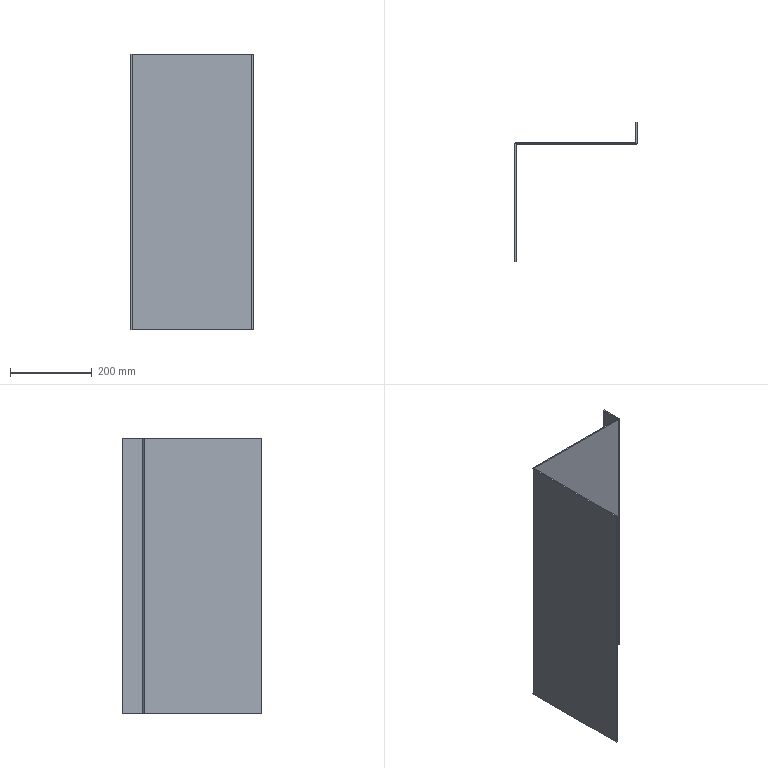Part | STEP file | E3-Metering stair tread 1-125 | 1 solid | 14 faces | box 299 x 340 x 674 mm | volume 1281653 mm3 | plane 10 | cylinder 4 | commonest cylinder face diameters 2 x2 8 x2
STEP:
#1=CARTESIAN_POINT('',(0.,0.,0.));
#2=DIRECTION('',(0.,0.,1.));
#3=DIRECTION('',(1.,0.,0.));
#4=AXIS2_PLACEMENT_3D('',#1,#2,#3);
#5=CARTESIAN_POINT('',(3.,1.,337.));
#6=VERTEX_POINT('',#5);
#7=CARTESIAN_POINT('',(3.,50.,337.));
#8=VERTEX_POINT('',#7);
#9=CARTESIAN_POINT('',(3.,1.,337.));
#10=DIRECTION('',(0.,1.,0.));
#11=VECTOR('',#10,1.);
#12=LINE('',#9,#11);
#13=CARTESIAN_POINT('',(3.,1.,-337.));
#14=DIRECTION('',(-1.,0.,0.));
#15=DIRECTION('',(0.,0.,-1.));
#16=AXIS2_PLACEMENT_3D('',#13,#14,#15);
#17=PLANE('',#16);
#18=CARTESIAN_POINT('',(-674.,0.));
#19=DIRECTION('',(0.,-1.));
#20=VECTOR('',#19,1.);
#21=LINE('',#18,#20);
#22=(GEOMETRIC_REPRESENTATION_CONTEXT(2)PARAMETRIC_REPRESENTATION_CONTEXT()REPRESENTATION_CONTEXT('',''));
#23=DEFINITIONAL_REPRESENTATION('',(#21),#22);
#24=PCURVE('',#17,#23);
#25=CARTESIAN_POINT('',(-1.,1.,337.));
#26=DIRECTION('',(0.,0.,-1.));
#27=DIRECTION('',(1.,0.,0.));
#28=AXIS2_PLACEMENT_3D('',#25,#26,#27);
#29=PLANE('',#28);
#30=CARTESIAN_POINT('',(4.,0.));
#31=DIRECTION('',(0.,-1.));
#32=VECTOR('',#31,1.);
#33=LINE('',#30,#32);
#34=(GEOMETRIC_REPRESENTATION_CONTEXT(2)PARAMETRIC_REPRESENTATION_CONTEXT()REPRESENTATION_CONTEXT('',''));
#35=DEFINITIONAL_REPRESENTATION('',(#33),#34);
#36=PCURVE('',#29,#35);
#37=SURFACE_CURVE('',#12,(#24,#36),.PCURVE_S1.);
#38=EDGE_CURVE('',#6,#8,#37,.T.);
#39=ORIENTED_EDGE('',*,*,#38,.F.);
#40=CARTESIAN_POINT('',(3.,1.,-337.));
#41=VERTEX_POINT('',#40);
#42=CARTESIAN_POINT('',(3.,1.,-337.));
#43=DIRECTION('',(0.,0.,1.));
#44=VECTOR('',#43,1.);
#45=LINE('',#42,#44);
#46=CARTESIAN_POINT('',(0.,0.));
#47=DIRECTION('',(-1.,0.));
#48=VECTOR('',#47,1.);
#49=LINE('',#46,#48);
#50=(GEOMETRIC_REPRESENTATION_CONTEXT(2)PARAMETRIC_REPRESENTATION_CONTEXT()REPRESENTATION_CONTEXT('',''));
#51=DEFINITIONAL_REPRESENTATION('',(#49),#50);
#52=PCURVE('',#17,#51);
#53=CARTESIAN_POINT('',(-1.,1.,-337.));
#54=DIRECTION('',(0.,0.,1.));
#55=DIRECTION('',(-1.,0.,0.));
#56=AXIS2_PLACEMENT_3D('',#53,#54,#55);
#57=CYLINDRICAL_SURFACE('',#56,4.);
#58=CARTESIAN_POINT('',(3.142,0.));
#59=DIRECTION('',(0.,1.));
#60=VECTOR('',#59,1.);
#61=LINE('',#58,#60);
#62=(GEOMETRIC_REPRESENTATION_CONTEXT(2)PARAMETRIC_REPRESENTATION_CONTEXT()REPRESENTATION_CONTEXT('',''));
#63=DEFINITIONAL_REPRESENTATION('',(#61),#62);
#64=PCURVE('',#57,#63);
#65=SURFACE_CURVE('',#45,(#52,#64),.PCURVE_S1.);
#66=EDGE_CURVE('',#41,#6,#65,.T.);
#67=ORIENTED_EDGE('',*,*,#66,.F.);
#68=CARTESIAN_POINT('',(3.,50.,-337.));
#69=VERTEX_POINT('',#68);
#70=CARTESIAN_POINT('',(3.,1.,-337.));
#71=DIRECTION('',(0.,1.,0.));
#72=VECTOR('',#71,1.);
#73=LINE('',#70,#72);
#74=CARTESIAN_POINT('',(0.,0.));
#75=DIRECTION('',(0.,-1.));
#76=VECTOR('',#75,1.);
#77=LINE('',#74,#76);
#78=(GEOMETRIC_REPRESENTATION_CONTEXT(2)PARAMETRIC_REPRESENTATION_CONTEXT()REPRESENTATION_CONTEXT('',''));
#79=DEFINITIONAL_REPRESENTATION('',(#77),#78);
#80=PCURVE('',#17,#79);
#81=CARTESIAN_POINT('',(-1.,1.,-337.));
#82=DIRECTION('',(0.,0.,-1.));
#83=DIRECTION('',(1.,0.,0.));
#84=AXIS2_PLACEMENT_3D('',#81,#82,#83);
#85=PLANE('',#84);
#86=CARTESIAN_POINT('',(4.,0.));
#87=DIRECTION('',(0.,-1.));
#88=VECTOR('',#87,1.);
#89=LINE('',#86,#88);
#90=(GEOMETRIC_REPRESENTATION_CONTEXT(2)PARAMETRIC_REPRESENTATION_CONTEXT()REPRESENTATION_CONTEXT('',''));
#91=DEFINITIONAL_REPRESENTATION('',(#89),#90);
#92=PCURVE('',#85,#91);
#93=SURFACE_CURVE('',#73,(#80,#92),.PCURVE_S1.);
#94=EDGE_CURVE('',#41,#69,#93,.T.);
#95=ORIENTED_EDGE('',*,*,#94,.T.);
#96=CARTESIAN_POINT('',(3.,50.,-337.));
#97=DIRECTION('',(0.,0.,1.));
#98=VECTOR('',#97,1.);
#99=LINE('',#96,#98);
#100=CARTESIAN_POINT('',(0.,-49.));
#101=DIRECTION('',(-1.,0.));
#102=VECTOR('',#101,1.);
#103=LINE('',#100,#102);
#104=(GEOMETRIC_REPRESENTATION_CONTEXT(2)PARAMETRIC_REPRESENTATION_CONTEXT()REPRESENTATION_CONTEXT('',''));
#105=DEFINITIONAL_REPRESENTATION('',(#103),#104);
#106=PCURVE('',#17,#105);
#107=CARTESIAN_POINT('',(0.,50.,-337.));
#108=DIRECTION('',(0.,1.,0.));
#109=DIRECTION('',(0.,0.,-1.));
#110=AXIS2_PLACEMENT_3D('',#107,#108,#109);
#111=PLANE('',#110);
#112=CARTESIAN_POINT('',(0.,-3.));
#113=DIRECTION('',(-1.,0.));
#114=VECTOR('',#113,1.);
#115=LINE('',#112,#114);
#116=(GEOMETRIC_REPRESENTATION_CONTEXT(2)PARAMETRIC_REPRESENTATION_CONTEXT()REPRESENTATION_CONTEXT('',''));
#117=DEFINITIONAL_REPRESENTATION('',(#115),#116);
#118=PCURVE('',#111,#117);
#119=SURFACE_CURVE('',#99,(#106,#118),.PCURVE_S1.);
#120=EDGE_CURVE('',#69,#8,#119,.T.);
#121=ORIENTED_EDGE('',*,*,#120,.T.);
#122=EDGE_LOOP('',(#39,#67,#95,#121));
#123=FACE_BOUND('',#122,.T.);
#124=ADVANCED_FACE('',(#123),#17,.F.);
#125=CARTESIAN_POINT('',(0.,50.,337.));
#126=VERTEX_POINT('',#125);
#127=CARTESIAN_POINT('',(0.,50.,337.));
#128=DIRECTION('',(1.,0.,0.));
#129=VECTOR('',#128,1.);
#130=LINE('',#127,#129);
#131=CARTESIAN_POINT('',(-674.,0.));
#132=DIRECTION('',(0.,-1.));
#133=VECTOR('',#132,1.);
#134=LINE('',#131,#133);
#135=(GEOMETRIC_REPRESENTATION_CONTEXT(2)PARAMETRIC_REPRESENTATION_CONTEXT()REPRESENTATION_CONTEXT('',''));
#136=DEFINITIONAL_REPRESENTATION('',(#134),#135);
#137=PCURVE('',#111,#136);
#138=CARTESIAN_POINT('',(1.,-49.));
#139=DIRECTION('',(1.,0.));
#140=VECTOR('',#139,1.);
#141=LINE('',#138,#140);
#142=(GEOMETRIC_REPRESENTATION_CONTEXT(2)PARAMETRIC_REPRESENTATION_CONTEXT()REPRESENTATION_CONTEXT('',''));
#143=DEFINITIONAL_REPRESENTATION('',(#141),#142);
#144=PCURVE('',#29,#143);
#145=SURFACE_CURVE('',#130,(#137,#144),.PCURVE_S1.);
#146=EDGE_CURVE('',#126,#8,#145,.T.);
#147=ORIENTED_EDGE('',*,*,#146,.T.);
#148=ORIENTED_EDGE('',*,*,#120,.F.);
#149=CARTESIAN_POINT('',(0.,50.,-337.));
#150=VERTEX_POINT('',#149);
#151=CARTESIAN_POINT('',(0.,50.,-337.));
#152=DIRECTION('',(1.,0.,0.));
#153=VECTOR('',#152,1.);
#154=LINE('',#151,#153);
#155=CARTESIAN_POINT('',(0.,0.));
#156=DIRECTION('',(0.,-1.));
#157=VECTOR('',#156,1.);
#158=LINE('',#155,#157);
#159=(GEOMETRIC_REPRESENTATION_CONTEXT(2)PARAMETRIC_REPRESENTATION_CONTEXT()REPRESENTATION_CONTEXT('',''));
#160=DEFINITIONAL_REPRESENTATION('',(#158),#159);
#161=PCURVE('',#111,#160);
#162=CARTESIAN_POINT('',(1.,-49.));
#163=DIRECTION('',(1.,0.));
#164=VECTOR('',#163,1.);
#165=LINE('',#162,#164);
#166=(GEOMETRIC_REPRESENTATION_CONTEXT(2)PARAMETRIC_REPRESENTATION_CONTEXT()REPRESENTATION_CONTEXT('',''));
#167=DEFINITIONAL_REPRESENTATION('',(#165),#166);
#168=PCURVE('',#85,#167);
#169=SURFACE_CURVE('',#154,(#161,#168),.PCURVE_S1.);
#170=EDGE_CURVE('',#150,#69,#169,.T.);
#171=ORIENTED_EDGE('',*,*,#170,.F.);
#172=CARTESIAN_POINT('',(0.,50.,-337.));
#173=DIRECTION('',(0.,0.,1.));
#174=VECTOR('',#173,1.);
#175=LINE('',#172,#174);
#176=CARTESIAN_POINT('',(0.,0.));
#177=DIRECTION('',(-1.,0.));
#178=VECTOR('',#177,1.);
#179=LINE('',#176,#178);
#180=(GEOMETRIC_REPRESENTATION_CONTEXT(2)PARAMETRIC_REPRESENTATION_CONTEXT()REPRESENTATION_CONTEXT('',''));
#181=DEFINITIONAL_REPRESENTATION('',(#179),#180);
#182=PCURVE('',#111,#181);
#183=CARTESIAN_POINT('',(0.,1.,-337.));
#184=DIRECTION('',(-1.,0.,0.));
#185=DIRECTION('',(0.,0.,-1.));
#186=AXIS2_PLACEMENT_3D('',#183,#184,#185);
#187=PLANE('',#186);
#188=CARTESIAN_POINT('',(0.,-49.));
#189=DIRECTION('',(-1.,0.));
#190=VECTOR('',#189,1.);
#191=LINE('',#188,#190);
#192=(GEOMETRIC_REPRESENTATION_CONTEXT(2)PARAMETRIC_REPRESENTATION_CONTEXT()REPRESENTATION_CONTEXT('',''));
#193=DEFINITIONAL_REPRESENTATION('',(#191),#192);
#194=PCURVE('',#187,#193);
#195=SURFACE_CURVE('',#175,(#182,#194),.PCURVE_S1.);
#196=EDGE_CURVE('',#150,#126,#195,.T.);
#197=ORIENTED_EDGE('',*,*,#196,.T.);
#198=EDGE_LOOP('',(#147,#148,#171,#197));
#199=FACE_BOUND('',#198,.T.);
#200=ADVANCED_FACE('',(#199),#111,.T.);
#201=CARTESIAN_POINT('',(0.,1.,337.));
#202=VERTEX_POINT('',#201);
#203=CARTESIAN_POINT('',(0.,1.,337.));
#204=DIRECTION('',(0.,1.,0.));
#205=VECTOR('',#204,1.);
#206=LINE('',#203,#205);
#207=CARTESIAN_POINT('',(-674.,0.));
#208=DIRECTION('',(0.,-1.));
#209=VECTOR('',#208,1.);
#210=LINE('',#207,#209);
#211=(GEOMETRIC_REPRESENTATION_CONTEXT(2)PARAMETRIC_REPRESENTATION_CONTEXT()REPRESENTATION_CONTEXT('',''));
#212=DEFINITIONAL_REPRESENTATION('',(#210),#211);
#213=PCURVE('',#187,#212);
#214=CARTESIAN_POINT('',(1.,0.));
#215=DIRECTION('',(0.,-1.));
#216=VECTOR('',#215,1.);
#217=LINE('',#214,#216);
#218=(GEOMETRIC_REPRESENTATION_CONTEXT(2)PARAMETRIC_REPRESENTATION_CONTEXT()REPRESENTATION_CONTEXT('',''));
#219=DEFINITIONAL_REPRESENTATION('',(#217),#218);
#220=PCURVE('',#29,#219);
#221=SURFACE_CURVE('',#206,(#213,#220),.PCURVE_S1.);
#222=EDGE_CURVE('',#202,#126,#221,.T.);
#223=ORIENTED_EDGE('',*,*,#222,.T.);
#224=ORIENTED_EDGE('',*,*,#196,.F.);
#225=CARTESIAN_POINT('',(0.,1.,-337.));
#226=VERTEX_POINT('',#225);
#227=CARTESIAN_POINT('',(0.,1.,-337.));
#228=DIRECTION('',(0.,1.,0.));
#229=VECTOR('',#228,1.);
#230=LINE('',#227,#229);
#231=CARTESIAN_POINT('',(0.,0.));
#232=DIRECTION('',(0.,-1.));
#233=VECTOR('',#232,1.);
#234=LINE('',#231,#233);
#235=(GEOMETRIC_REPRESENTATION_CONTEXT(2)PARAMETRIC_REPRESENTATION_CONTEXT()REPRESENTATION_CONTEXT('',''));
#236=DEFINITIONAL_REPRESENTATION('',(#234),#235);
#237=PCURVE('',#187,#236);
#238=CARTESIAN_POINT('',(1.,0.));
#239=DIRECTION('',(0.,-1.));
#240=VECTOR('',#239,1.);
#241=LINE('',#238,#240);
#242=(GEOMETRIC_REPRESENTATION_CONTEXT(2)PARAMETRIC_REPRESENTATION_CONTEXT()REPRESENTATION_CONTEXT('',''));
#243=DEFINITIONAL_REPRESENTATION('',(#241),#242);
#244=PCURVE('',#85,#243);
#245=SURFACE_CURVE('',#230,(#237,#244),.PCURVE_S1.);
#246=EDGE_CURVE('',#226,#150,#245,.T.);
#247=ORIENTED_EDGE('',*,*,#246,.F.);
#248=CARTESIAN_POINT('',(0.,1.,-337.));
#249=DIRECTION('',(0.,0.,1.));
#250=VECTOR('',#249,1.);
#251=LINE('',#248,#250);
#252=CARTESIAN_POINT('',(0.,0.));
#253=DIRECTION('',(-1.,0.));
#254=VECTOR('',#253,1.);
#255=LINE('',#252,#254);
#256=(GEOMETRIC_REPRESENTATION_CONTEXT(2)PARAMETRIC_REPRESENTATION_CONTEXT()REPRESENTATION_CONTEXT('',''));
#257=DEFINITIONAL_REPRESENTATION('',(#255),#256);
#258=PCURVE('',#187,#257);
#259=CARTESIAN_POINT('',(-1.,1.,-337.));
#260=DIRECTION('',(0.,0.,1.));
#261=DIRECTION('',(-1.,0.,0.));
#262=AXIS2_PLACEMENT_3D('',#259,#260,#261);
#263=CYLINDRICAL_SURFACE('',#262,1.);
#264=CARTESIAN_POINT('',(3.142,0.));
#265=DIRECTION('',(0.,1.));
#266=VECTOR('',#265,1.);
#267=LINE('',#264,#266);
#268=(GEOMETRIC_REPRESENTATION_CONTEXT(2)PARAMETRIC_REPRESENTATION_CONTEXT()REPRESENTATION_CONTEXT('',''));
#269=DEFINITIONAL_REPRESENTATION('',(#267),#268);
#270=PCURVE('',#263,#269);
#271=SURFACE_CURVE('',#251,(#258,#270),.PCURVE_S1.);
#272=EDGE_CURVE('',#226,#202,#271,.T.);
#273=ORIENTED_EDGE('',*,*,#272,.T.);
#274=EDGE_LOOP('',(#223,#224,#247,#273));
#275=FACE_BOUND('',#274,.T.);
#276=ADVANCED_FACE('',(#275),#187,.T.);
#277=CARTESIAN_POINT('',(-1.,0.,-337.));
#278=VERTEX_POINT('',#277);
#279=CARTESIAN_POINT('',(-1.,0.,337.));
#280=VERTEX_POINT('',#279);
#281=CARTESIAN_POINT('',(-1.,0.,-337.));
#282=DIRECTION('',(0.,0.,1.));
#283=VECTOR('',#282,1.);
#284=LINE('',#281,#283);
#285=CARTESIAN_POINT('',(1.571,0.));
#286=DIRECTION('',(0.,1.));
#287=VECTOR('',#286,1.);
#288=LINE('',#285,#287);
#289=(GEOMETRIC_REPRESENTATION_CONTEXT(2)PARAMETRIC_REPRESENTATION_CONTEXT()REPRESENTATION_CONTEXT('',''));
#290=DEFINITIONAL_REPRESENTATION('',(#288),#289);
#291=PCURVE('',#263,#290);
#292=CARTESIAN_POINT('',(-292.,0.,-337.));
#293=DIRECTION('',(0.,1.,0.));
#294=DIRECTION('',(0.,0.,-1.));
#295=AXIS2_PLACEMENT_3D('',#292,#293,#294);
#296=PLANE('',#295);
#297=CARTESIAN_POINT('',(0.,-291.));
#298=DIRECTION('',(-1.,0.));
#299=VECTOR('',#298,1.);
#300=LINE('',#297,#299);
#301=(GEOMETRIC_REPRESENTATION_CONTEXT(2)PARAMETRIC_REPRESENTATION_CONTEXT()REPRESENTATION_CONTEXT('',''));
#302=DEFINITIONAL_REPRESENTATION('',(#300),#301);
#303=PCURVE('',#296,#302);
#304=SURFACE_CURVE('',#284,(#291,#303),.PCURVE_S1.);
#305=EDGE_CURVE('',#278,#280,#304,.T.);
#306=ORIENTED_EDGE('',*,*,#305,.F.);
#307=CARTESIAN_POINT('',(-1.,1.,-337.));
#308=DIRECTION('',(0.,0.,1.));
#309=DIRECTION('',(1.,0.,0.));
#310=AXIS2_PLACEMENT_3D('',#307,#308,#309);
#311=CIRCLE('',#310,1.);
#312=CARTESIAN_POINT('',(-3.142,0.));
#313=DIRECTION('',(1.,0.));
#314=VECTOR('',#313,1.);
#315=LINE('',#312,#314);
#316=(GEOMETRIC_REPRESENTATION_CONTEXT(2)PARAMETRIC_REPRESENTATION_CONTEXT()REPRESENTATION_CONTEXT('',''));
#317=DEFINITIONAL_REPRESENTATION('',(#315),#316);
#318=PCURVE('',#263,#317);
#319=CARTESIAN_POINT('',(1.,0.));
#320=CARTESIAN_POINT('',(1.,-1.732));
#321=CARTESIAN_POINT('',(-0.5,-0.866));
#322=CARTESIAN_POINT('',(-2.,0.));
#323=CARTESIAN_POINT('',(-0.5,0.866));
#324=CARTESIAN_POINT('',(1.,1.732));
#325=CARTESIAN_POINT('',(1.,0.));
#326=(BOUNDED_CURVE()B_SPLINE_CURVE(2,(#319,#320,#321,#322,#323,#324,#325),.UNSPECIFIED.,.T.,.F.)B_SPLINE_CURVE_WITH_KNOTS((1,2,2,2,2,1),(-2.094,0.,2.094,4.189,6.283,8.378),.UNSPECIFIED.)CURVE()GEOMETRIC_REPRESENTATION_ITEM()RATIONAL_B_SPLINE_CURVE((1.,0.5,1.,0.5,1.,0.5,1.))REPRESENTATION_ITEM(''));
#327=(GEOMETRIC_REPRESENTATION_CONTEXT(2)PARAMETRIC_REPRESENTATION_CONTEXT()REPRESENTATION_CONTEXT('',''));
#328=DEFINITIONAL_REPRESENTATION('',(#326),#327);
#329=PCURVE('',#85,#328);
#330=SURFACE_CURVE('',#311,(#318,#329),.PCURVE_S1.);
#331=EDGE_CURVE('',#278,#226,#330,.T.);
#332=ORIENTED_EDGE('',*,*,#331,.T.);
#333=ORIENTED_EDGE('',*,*,#272,.T.);
#334=CARTESIAN_POINT('',(-1.,1.,337.));
#335=DIRECTION('',(0.,0.,1.));
#336=DIRECTION('',(1.,0.,0.));
#337=AXIS2_PLACEMENT_3D('',#334,#335,#336);
#338=CIRCLE('',#337,1.);
#339=CARTESIAN_POINT('',(-3.142,674.));
#340=DIRECTION('',(1.,0.));
#341=VECTOR('',#340,1.);
#342=LINE('',#339,#341);
#343=(GEOMETRIC_REPRESENTATION_CONTEXT(2)PARAMETRIC_REPRESENTATION_CONTEXT()REPRESENTATION_CONTEXT('',''));
#344=DEFINITIONAL_REPRESENTATION('',(#342),#343);
#345=PCURVE('',#263,#344);
#346=CARTESIAN_POINT('',(1.,0.));
#347=CARTESIAN_POINT('',(1.,-1.732));
#348=CARTESIAN_POINT('',(-0.5,-0.866));
#349=CARTESIAN_POINT('',(-2.,0.));
#350=CARTESIAN_POINT('',(-0.5,0.866));
#351=CARTESIAN_POINT('',(1.,1.732));
#352=CARTESIAN_POINT('',(1.,0.));
#353=(BOUNDED_CURVE()B_SPLINE_CURVE(2,(#346,#347,#348,#349,#350,#351,#352),.UNSPECIFIED.,.T.,.F.)B_SPLINE_CURVE_WITH_KNOTS((1,2,2,2,2,1),(-2.094,0.,2.094,4.189,6.283,8.378),.UNSPECIFIED.)CURVE()GEOMETRIC_REPRESENTATION_ITEM()RATIONAL_B_SPLINE_CURVE((1.,0.5,1.,0.5,1.,0.5,1.))REPRESENTATION_ITEM(''));
#354=(GEOMETRIC_REPRESENTATION_CONTEXT(2)PARAMETRIC_REPRESENTATION_CONTEXT()REPRESENTATION_CONTEXT('',''));
#355=DEFINITIONAL_REPRESENTATION('',(#353),#354);
#356=PCURVE('',#29,#355);
#357=SURFACE_CURVE('',#338,(#345,#356),.PCURVE_S1.);
#358=EDGE_CURVE('',#280,#202,#357,.T.);
#359=ORIENTED_EDGE('',*,*,#358,.F.);
#360=EDGE_LOOP('',(#306,#332,#333,#359));
#361=FACE_BOUND('',#360,.F.);
#362=ADVANCED_FACE('',(#361),#263,.F.);
#363=CARTESIAN_POINT('',(-292.,0.,337.));
#364=VERTEX_POINT('',#363);
#365=CARTESIAN_POINT('',(-292.,0.,337.));
#366=DIRECTION('',(1.,0.,0.));
#367=VECTOR('',#366,1.);
#368=LINE('',#365,#367);
#369=CARTESIAN_POINT('',(-674.,0.));
#370=DIRECTION('',(0.,-1.));
#371=VECTOR('',#370,1.);
#372=LINE('',#369,#371);
#373=(GEOMETRIC_REPRESENTATION_CONTEXT(2)PARAMETRIC_REPRESENTATION_CONTEXT()REPRESENTATION_CONTEXT('',''));
#374=DEFINITIONAL_REPRESENTATION('',(#372),#373);
#375=PCURVE('',#296,#374);
#376=CARTESIAN_POINT('',(-291.,1.));
#377=DIRECTION('',(1.,0.));
#378=VECTOR('',#377,1.);
#379=LINE('',#376,#378);
#380=(GEOMETRIC_REPRESENTATION_CONTEXT(2)PARAMETRIC_REPRESENTATION_CONTEXT()REPRESENTATION_CONTEXT('',''));
#381=DEFINITIONAL_REPRESENTATION('',(#379),#380);
#382=PCURVE('',#29,#381);
#383=SURFACE_CURVE('',#368,(#375,#382),.PCURVE_S1.);
#384=EDGE_CURVE('',#364,#280,#383,.T.);
#385=ORIENTED_EDGE('',*,*,#384,.T.);
#386=ORIENTED_EDGE('',*,*,#305,.F.);
#387=CARTESIAN_POINT('',(-292.,0.,-337.));
#388=VERTEX_POINT('',#387);
#389=CARTESIAN_POINT('',(-292.,0.,-337.));
#390=DIRECTION('',(1.,0.,0.));
#391=VECTOR('',#390,1.);
#392=LINE('',#389,#391);
#393=CARTESIAN_POINT('',(0.,0.));
#394=DIRECTION('',(0.,-1.));
#395=VECTOR('',#394,1.);
#396=LINE('',#393,#395);
#397=(GEOMETRIC_REPRESENTATION_CONTEXT(2)PARAMETRIC_REPRESENTATION_CONTEXT()REPRESENTATION_CONTEXT('',''));
#398=DEFINITIONAL_REPRESENTATION('',(#396),#397);
#399=PCURVE('',#296,#398);
#400=CARTESIAN_POINT('',(-291.,1.));
#401=DIRECTION('',(1.,0.));
#402=VECTOR('',#401,1.);
#403=LINE('',#400,#402);
#404=(GEOMETRIC_REPRESENTATION_CONTEXT(2)PARAMETRIC_REPRESENTATION_CONTEXT()REPRESENTATION_CONTEXT('',''));
#405=DEFINITIONAL_REPRESENTATION('',(#403),#404);
#406=PCURVE('',#85,#405);
#407=SURFACE_CURVE('',#392,(#399,#406),.PCURVE_S1.);
#408=EDGE_CURVE('',#388,#278,#407,.T.);
#409=ORIENTED_EDGE('',*,*,#408,.F.);
#410=CARTESIAN_POINT('',(-292.,0.,-337.));
#411=DIRECTION('',(0.,0.,1.));
#412=VECTOR('',#411,1.);
#413=LINE('',#410,#412);
#414=CARTESIAN_POINT('',(0.,0.));
#415=DIRECTION('',(-1.,0.));
#416=VECTOR('',#415,1.);
#417=LINE('',#414,#416);
#418=(GEOMETRIC_REPRESENTATION_CONTEXT(2)PARAMETRIC_REPRESENTATION_CONTEXT()REPRESENTATION_CONTEXT('',''));
#419=DEFINITIONAL_REPRESENTATION('',(#417),#418);
#420=PCURVE('',#296,#419);
#421=CARTESIAN_POINT('',(-292.,-4.,-337.));
#422=DIRECTION('',(0.,0.,1.));
#423=DIRECTION('',(-1.,0.,0.));
#424=AXIS2_PLACEMENT_3D('',#421,#422,#423);
#425=CYLINDRICAL_SURFACE('',#424,4.);
#426=CARTESIAN_POINT('',(4.712,0.));
#427=DIRECTION('',(0.,1.));
#428=VECTOR('',#427,1.);
#429=LINE('',#426,#428);
#430=(GEOMETRIC_REPRESENTATION_CONTEXT(2)PARAMETRIC_REPRESENTATION_CONTEXT()REPRESENTATION_CONTEXT('',''));
#431=DEFINITIONAL_REPRESENTATION('',(#429),#430);
#432=PCURVE('',#425,#431);
#433=SURFACE_CURVE('',#413,(#420,#432),.PCURVE_S1.);
#434=EDGE_CURVE('',#388,#364,#433,.T.);
#435=ORIENTED_EDGE('',*,*,#434,.T.);
#436=EDGE_LOOP('',(#385,#386,#409,#435));
#437=FACE_BOUND('',#436,.T.);
#438=ADVANCED_FACE('',(#437),#296,.T.);
#439=CARTESIAN_POINT('',(-296.,-4.,337.));
#440=VERTEX_POINT('',#439);
#441=CARTESIAN_POINT('',(-292.,-4.,337.));
#442=DIRECTION('',(0.,0.,-1.));
#443=DIRECTION('',(1.,0.,0.));
#444=AXIS2_PLACEMENT_3D('',#441,#442,#443);
#445=CIRCLE('',#444,4.);
#446=CARTESIAN_POINT('',(9.425,674.));
#447=DIRECTION('',(-1.,0.));
#448=VECTOR('',#447,1.);
#449=LINE('',#446,#448);
#450=(GEOMETRIC_REPRESENTATION_CONTEXT(2)PARAMETRIC_REPRESENTATION_CONTEXT()REPRESENTATION_CONTEXT('',''));
#451=DEFINITIONAL_REPRESENTATION('',(#449),#450);
#452=PCURVE('',#425,#451);
#453=CARTESIAN_POINT('',(-291.,5.));
#454=DIRECTION('',(1.,0.));
#455=AXIS2_PLACEMENT_2D('',#453,#454);
#456=CIRCLE('',#455,4.);
#457=(GEOMETRIC_REPRESENTATION_CONTEXT(2)PARAMETRIC_REPRESENTATION_CONTEXT()REPRESENTATION_CONTEXT('',''));
#458=DEFINITIONAL_REPRESENTATION('',(#456),#457);
#459=PCURVE('',#29,#458);
#460=SURFACE_CURVE('',#445,(#452,#459),.PCURVE_S1.);
#461=EDGE_CURVE('',#440,#364,#460,.T.);
#462=ORIENTED_EDGE('',*,*,#461,.T.);
#463=ORIENTED_EDGE('',*,*,#434,.F.);
#464=CARTESIAN_POINT('',(-296.,-4.,-337.));
#465=VERTEX_POINT('',#464);
#466=CARTESIAN_POINT('',(-292.,-4.,-337.));
#467=DIRECTION('',(0.,0.,-1.));
#468=DIRECTION('',(1.,0.,0.));
#469=AXIS2_PLACEMENT_3D('',#466,#467,#468);
#470=CIRCLE('',#469,4.);
#471=CARTESIAN_POINT('',(9.425,0.));
#472=DIRECTION('',(-1.,0.));
#473=VECTOR('',#472,1.);
#474=LINE('',#471,#473);
#475=(GEOMETRIC_REPRESENTATION_CONTEXT(2)PARAMETRIC_REPRESENTATION_CONTEXT()REPRESENTATION_CONTEXT('',''));
#476=DEFINITIONAL_REPRESENTATION('',(#474),#475);
#477=PCURVE('',#425,#476);
#478=CARTESIAN_POINT('',(-291.,5.));
#479=DIRECTION('',(1.,0.));
#480=AXIS2_PLACEMENT_2D('',#478,#479);
#481=CIRCLE('',#480,4.);
#482=(GEOMETRIC_REPRESENTATION_CONTEXT(2)PARAMETRIC_REPRESENTATION_CONTEXT()REPRESENTATION_CONTEXT('',''));
#483=DEFINITIONAL_REPRESENTATION('',(#481),#482);
#484=PCURVE('',#85,#483);
#485=SURFACE_CURVE('',#470,(#477,#484),.PCURVE_S1.);
#486=EDGE_CURVE('',#465,#388,#485,.T.);
#487=ORIENTED_EDGE('',*,*,#486,.F.);
#488=CARTESIAN_POINT('',(-296.,-4.,-337.));
#489=DIRECTION('',(0.,0.,1.));
#490=VECTOR('',#489,1.);
#491=LINE('',#488,#490);
#492=CARTESIAN_POINT('',(6.283,0.));
#493=DIRECTION('',(0.,1.));
#494=VECTOR('',#493,1.);
#495=LINE('',#492,#494);
#496=(GEOMETRIC_REPRESENTATION_CONTEXT(2)PARAMETRIC_REPRESENTATION_CONTEXT()REPRESENTATION_CONTEXT('',''));
#497=DEFINITIONAL_REPRESENTATION('',(#495),#496);
#498=PCURVE('',#425,#497);
#499=CARTESIAN_POINT('',(-296.,-4.,-337.));
#500=DIRECTION('',(-1.,0.,0.));
#501=DIRECTION('',(0.,0.,-1.));
#502=AXIS2_PLACEMENT_3D('',#499,#500,#501);
#503=PLANE('',#502);
#504=CARTESIAN_POINT('',(0.,0.));
#505=DIRECTION('',(-1.,0.));
#506=VECTOR('',#505,1.);
#507=LINE('',#504,#506);
#508=(GEOMETRIC_REPRESENTATION_CONTEXT(2)PARAMETRIC_REPRESENTATION_CONTEXT()REPRESENTATION_CONTEXT('',''));
#509=DEFINITIONAL_REPRESENTATION('',(#507),#508);
#510=PCURVE('',#503,#509);
#511=SURFACE_CURVE('',#491,(#498,#510),.PCURVE_S1.);
#512=EDGE_CURVE('',#465,#440,#511,.T.);
#513=ORIENTED_EDGE('',*,*,#512,.T.);
#514=EDGE_LOOP('',(#462,#463,#487,#513));
#515=FACE_BOUND('',#514,.T.);
#516=ADVANCED_FACE('',(#515),#425,.T.);
#517=CARTESIAN_POINT('',(-296.,-290.,337.));
#518=VERTEX_POINT('',#517);
#519=CARTESIAN_POINT('',(-296.,-4.,337.));
#520=DIRECTION('',(0.,1.,0.));
#521=VECTOR('',#520,1.);
#522=LINE('',#519,#521);
#523=CARTESIAN_POINT('',(-674.,0.));
#524=DIRECTION('',(0.,-1.));
#525=VECTOR('',#524,1.);
#526=LINE('',#523,#525);
#527=(GEOMETRIC_REPRESENTATION_CONTEXT(2)PARAMETRIC_REPRESENTATION_CONTEXT()REPRESENTATION_CONTEXT('',''));
#528=DEFINITIONAL_REPRESENTATION('',(#526),#527);
#529=PCURVE('',#503,#528);
#530=CARTESIAN_POINT('',(-295.,5.));
#531=DIRECTION('',(0.,-1.));
#532=VECTOR('',#531,1.);
#533=LINE('',#530,#532);
#534=(GEOMETRIC_REPRESENTATION_CONTEXT(2)PARAMETRIC_REPRESENTATION_CONTEXT()REPRESENTATION_CONTEXT('',''));
#535=DEFINITIONAL_REPRESENTATION('',(#533),#534);
#536=PCURVE('',#29,#535);
#537=SURFACE_CURVE('',#522,(#529,#536),.PCURVE_S1.);
#538=EDGE_CURVE('',#518,#440,#537,.T.);
#539=ORIENTED_EDGE('',*,*,#538,.T.);
#540=ORIENTED_EDGE('',*,*,#512,.F.);
#541=CARTESIAN_POINT('',(-296.,-290.,-337.));
#542=VERTEX_POINT('',#541);
#543=CARTESIAN_POINT('',(-296.,-4.,-337.));
#544=DIRECTION('',(0.,1.,0.));
#545=VECTOR('',#544,1.);
#546=LINE('',#543,#545);
#547=CARTESIAN_POINT('',(0.,0.));
#548=DIRECTION('',(0.,-1.));
#549=VECTOR('',#548,1.);
#550=LINE('',#547,#549);
#551=(GEOMETRIC_REPRESENTATION_CONTEXT(2)PARAMETRIC_REPRESENTATION_CONTEXT()REPRESENTATION_CONTEXT('',''));
#552=DEFINITIONAL_REPRESENTATION('',(#550),#551);
#553=PCURVE('',#503,#552);
#554=CARTESIAN_POINT('',(-295.,5.));
#555=DIRECTION('',(0.,-1.));
#556=VECTOR('',#555,1.);
#557=LINE('',#554,#556);
#558=(GEOMETRIC_REPRESENTATION_CONTEXT(2)PARAMETRIC_REPRESENTATION_CONTEXT()REPRESENTATION_CONTEXT('',''));
#559=DEFINITIONAL_REPRESENTATION('',(#557),#558);
#560=PCURVE('',#85,#559);
#561=SURFACE_CURVE('',#546,(#553,#560),.PCURVE_S1.);
#562=EDGE_CURVE('',#542,#465,#561,.T.);
#563=ORIENTED_EDGE('',*,*,#562,.F.);
#564=CARTESIAN_POINT('',(-296.,-290.,-337.));
#565=DIRECTION('',(0.,0.,1.));
#566=VECTOR('',#565,1.);
#567=LINE('',#564,#566);
#568=CARTESIAN_POINT('',(0.,286.));
#569=DIRECTION('',(-1.,0.));
#570=VECTOR('',#569,1.);
#571=LINE('',#568,#570);
#572=(GEOMETRIC_REPRESENTATION_CONTEXT(2)PARAMETRIC_REPRESENTATION_CONTEXT()REPRESENTATION_CONTEXT('',''));
#573=DEFINITIONAL_REPRESENTATION('',(#571),#572);
#574=PCURVE('',#503,#573);
#575=CARTESIAN_POINT('',(-293.,-290.,-337.));
#576=DIRECTION('',(0.,-1.,0.));
#577=DIRECTION('',(0.,0.,1.));
#578=AXIS2_PLACEMENT_3D('',#575,#576,#577);
#579=PLANE('',#578);
#580=CARTESIAN_POINT('',(0.,3.));
#581=DIRECTION('',(1.,0.));
#582=VECTOR('',#581,1.);
#583=LINE('',#580,#582);
#584=(GEOMETRIC_REPRESENTATION_CONTEXT(2)PARAMETRIC_REPRESENTATION_CONTEXT()REPRESENTATION_CONTEXT('',''));
#585=DEFINITIONAL_REPRESENTATION('',(#583),#584);
#586=PCURVE('',#579,#585);
#587=SURFACE_CURVE('',#567,(#574,#586),.PCURVE_S1.);
#588=EDGE_CURVE('',#542,#518,#587,.T.);
#589=ORIENTED_EDGE('',*,*,#588,.T.);
#590=EDGE_LOOP('',(#539,#540,#563,#589));
#591=FACE_BOUND('',#590,.T.);
#592=ADVANCED_FACE('',(#591),#503,.T.);
#593=CARTESIAN_POINT('',(-293.,-290.,337.));
#594=VERTEX_POINT('',#593);
#595=CARTESIAN_POINT('',(-293.,-290.,337.));
#596=DIRECTION('',(-1.,0.,0.));
#597=VECTOR('',#596,1.);
#598=LINE('',#595,#597);
#599=CARTESIAN_POINT('',(674.,0.));
#600=DIRECTION('',(0.,1.));
#601=VECTOR('',#600,1.);
#602=LINE('',#599,#601);
#603=(GEOMETRIC_REPRESENTATION_CONTEXT(2)PARAMETRIC_REPRESENTATION_CONTEXT()REPRESENTATION_CONTEXT('',''));
#604=DEFINITIONAL_REPRESENTATION('',(#602),#603);
#605=PCURVE('',#579,#604);
#606=CARTESIAN_POINT('',(-292.,291.));
#607=DIRECTION('',(-1.,0.));
#608=VECTOR('',#607,1.);
#609=LINE('',#606,#608);
#610=(GEOMETRIC_REPRESENTATION_CONTEXT(2)PARAMETRIC_REPRESENTATION_CONTEXT()REPRESENTATION_CONTEXT('',''));
#611=DEFINITIONAL_REPRESENTATION('',(#609),#610);
#612=PCURVE('',#29,#611);
#613=SURFACE_CURVE('',#598,(#605,#612),.PCURVE_S1.);
#614=EDGE_CURVE('',#594,#518,#613,.T.);
#615=ORIENTED_EDGE('',*,*,#614,.T.);
#616=ORIENTED_EDGE('',*,*,#588,.F.);
#617=CARTESIAN_POINT('',(-293.,-290.,-337.));
#618=VERTEX_POINT('',#617);
#619=CARTESIAN_POINT('',(-293.,-290.,-337.));
#620=DIRECTION('',(-1.,0.,0.));
#621=VECTOR('',#620,1.);
#622=LINE('',#619,#621);
#623=CARTESIAN_POINT('',(0.,0.));
#624=DIRECTION('',(0.,1.));
#625=VECTOR('',#624,1.);
#626=LINE('',#623,#625);
#627=(GEOMETRIC_REPRESENTATION_CONTEXT(2)PARAMETRIC_REPRESENTATION_CONTEXT()REPRESENTATION_CONTEXT('',''));
#628=DEFINITIONAL_REPRESENTATION('',(#626),#627);
#629=PCURVE('',#579,#628);
#630=CARTESIAN_POINT('',(-292.,291.));
#631=DIRECTION('',(-1.,0.));
#632=VECTOR('',#631,1.);
#633=LINE('',#630,#632);
#634=(GEOMETRIC_REPRESENTATION_CONTEXT(2)PARAMETRIC_REPRESENTATION_CONTEXT()REPRESENTATION_CONTEXT('',''));
#635=DEFINITIONAL_REPRESENTATION('',(#633),#634);
#636=PCURVE('',#85,#635);
#637=SURFACE_CURVE('',#622,(#629,#636),.PCURVE_S1.);
#638=EDGE_CURVE('',#618,#542,#637,.T.);
#639=ORIENTED_EDGE('',*,*,#638,.F.);
#640=CARTESIAN_POINT('',(-293.,-290.,-337.));
#641=DIRECTION('',(0.,0.,1.));
#642=VECTOR('',#641,1.);
#643=LINE('',#640,#642);
#644=CARTESIAN_POINT('',(0.,0.));
#645=DIRECTION('',(1.,0.));
#646=VECTOR('',#645,1.);
#647=LINE('',#644,#646);
#648=(GEOMETRIC_REPRESENTATION_CONTEXT(2)PARAMETRIC_REPRESENTATION_CONTEXT()REPRESENTATION_CONTEXT('',''));
#649=DEFINITIONAL_REPRESENTATION('',(#647),#648);
#650=PCURVE('',#579,#649);
#651=CARTESIAN_POINT('',(-293.,-4.,-337.));
#652=DIRECTION('',(-1.,0.,0.));
#653=DIRECTION('',(0.,0.,-1.));
#654=AXIS2_PLACEMENT_3D('',#651,#652,#653);
#655=PLANE('',#654);
#656=CARTESIAN_POINT('',(0.,286.));
#657=DIRECTION('',(-1.,0.));
#658=VECTOR('',#657,1.);
#659=LINE('',#656,#658);
#660=(GEOMETRIC_REPRESENTATION_CONTEXT(2)PARAMETRIC_REPRESENTATION_CONTEXT()REPRESENTATION_CONTEXT('',''));
#661=DEFINITIONAL_REPRESENTATION('',(#659),#660);
#662=PCURVE('',#655,#661);
#663=SURFACE_CURVE('',#643,(#650,#662),.PCURVE_S1.);
#664=EDGE_CURVE('',#618,#594,#663,.T.);
#665=ORIENTED_EDGE('',*,*,#664,.T.);
#666=EDGE_LOOP('',(#615,#616,#639,#665));
#667=FACE_BOUND('',#666,.T.);
#668=ADVANCED_FACE('',(#667),#579,.T.);
#669=CARTESIAN_POINT('',(-293.,-4.,337.));
#670=VERTEX_POINT('',#669);
#671=CARTESIAN_POINT('',(-293.,-4.,337.));
#672=DIRECTION('',(0.,1.,0.));
#673=VECTOR('',#672,1.);
#674=LINE('',#671,#673);
#675=CARTESIAN_POINT('',(-674.,0.));
#676=DIRECTION('',(0.,-1.));
#677=VECTOR('',#676,1.);
#678=LINE('',#675,#677);
#679=(GEOMETRIC_REPRESENTATION_CONTEXT(2)PARAMETRIC_REPRESENTATION_CONTEXT()REPRESENTATION_CONTEXT('',''));
#680=DEFINITIONAL_REPRESENTATION('',(#678),#679);
#681=PCURVE('',#655,#680);
#682=CARTESIAN_POINT('',(-292.,5.));
#683=DIRECTION('',(0.,-1.));
#684=VECTOR('',#683,1.);
#685=LINE('',#682,#684);
#686=(GEOMETRIC_REPRESENTATION_CONTEXT(2)PARAMETRIC_REPRESENTATION_CONTEXT()REPRESENTATION_CONTEXT('',''));
#687=DEFINITIONAL_REPRESENTATION('',(#685),#686);
#688=PCURVE('',#29,#687);
#689=SURFACE_CURVE('',#674,(#681,#688),.PCURVE_S1.);
#690=EDGE_CURVE('',#594,#670,#689,.T.);
#691=ORIENTED_EDGE('',*,*,#690,.F.);
#692=ORIENTED_EDGE('',*,*,#664,.F.);
#693=CARTESIAN_POINT('',(-293.,-4.,-337.));
#694=VERTEX_POINT('',#693);
#695=CARTESIAN_POINT('',(-293.,-4.,-337.));
#696=DIRECTION('',(0.,1.,0.));
#697=VECTOR('',#696,1.);
#698=LINE('',#695,#697);
#699=CARTESIAN_POINT('',(0.,0.));
#700=DIRECTION('',(0.,-1.));
#701=VECTOR('',#700,1.);
#702=LINE('',#699,#701);
#703=(GEOMETRIC_REPRESENTATION_CONTEXT(2)PARAMETRIC_REPRESENTATION_CONTEXT()REPRESENTATION_CONTEXT('',''));
#704=DEFINITIONAL_REPRESENTATION('',(#702),#703);
#705=PCURVE('',#655,#704);
#706=CARTESIAN_POINT('',(-292.,5.));
#707=DIRECTION('',(0.,-1.));
#708=VECTOR('',#707,1.);
#709=LINE('',#706,#708);
#710=(GEOMETRIC_REPRESENTATION_CONTEXT(2)PARAMETRIC_REPRESENTATION_CONTEXT()REPRESENTATION_CONTEXT('',''));
#711=DEFINITIONAL_REPRESENTATION('',(#709),#710);
#712=PCURVE('',#85,#711);
#713=SURFACE_CURVE('',#698,(#705,#712),.PCURVE_S1.);
#714=EDGE_CURVE('',#618,#694,#713,.T.);
#715=ORIENTED_EDGE('',*,*,#714,.T.);
#716=CARTESIAN_POINT('',(-293.,-4.,-337.));
#717=DIRECTION('',(0.,0.,1.));
#718=VECTOR('',#717,1.);
#719=LINE('',#716,#718);
#720=CARTESIAN_POINT('',(0.,0.));
#721=DIRECTION('',(-1.,0.));
#722=VECTOR('',#721,1.);
#723=LINE('',#720,#722);
#724=(GEOMETRIC_REPRESENTATION_CONTEXT(2)PARAMETRIC_REPRESENTATION_CONTEXT()REPRESENTATION_CONTEXT('',''));
#725=DEFINITIONAL_REPRESENTATION('',(#723),#724);
#726=PCURVE('',#655,#725);
#727=CARTESIAN_POINT('',(-292.,-4.,-337.));
#728=DIRECTION('',(0.,0.,1.));
#729=DIRECTION('',(-1.,0.,0.));
#730=AXIS2_PLACEMENT_3D('',#727,#728,#729);
#731=CYLINDRICAL_SURFACE('',#730,1.);
#732=CARTESIAN_POINT('',(6.283,0.));
#733=DIRECTION('',(0.,1.));
#734=VECTOR('',#733,1.);
#735=LINE('',#732,#734);
#736=(GEOMETRIC_REPRESENTATION_CONTEXT(2)PARAMETRIC_REPRESENTATION_CONTEXT()REPRESENTATION_CONTEXT('',''));
#737=DEFINITIONAL_REPRESENTATION('',(#735),#736);
#738=PCURVE('',#731,#737);
#739=SURFACE_CURVE('',#719,(#726,#738),.PCURVE_S1.);
#740=EDGE_CURVE('',#694,#670,#739,.T.);
#741=ORIENTED_EDGE('',*,*,#740,.T.);
#742=EDGE_LOOP('',(#691,#692,#715,#741));
#743=FACE_BOUND('',#742,.T.);
#744=ADVANCED_FACE('',(#743),#655,.F.);
#745=CARTESIAN_POINT('',(-292.,-3.,-337.));
#746=VERTEX_POINT('',#745);
#747=CARTESIAN_POINT('',(-292.,-3.,337.));
#748=VERTEX_POINT('',#747);
#749=CARTESIAN_POINT('',(-292.,-3.,-337.));
#750=DIRECTION('',(0.,0.,1.));
#751=VECTOR('',#750,1.);
#752=LINE('',#749,#751);
#753=CARTESIAN_POINT('',(4.712,0.));
#754=DIRECTION('',(0.,1.));
#755=VECTOR('',#754,1.);
#756=LINE('',#753,#755);
#757=(GEOMETRIC_REPRESENTATION_CONTEXT(2)PARAMETRIC_REPRESENTATION_CONTEXT()REPRESENTATION_CONTEXT('',''));
#758=DEFINITIONAL_REPRESENTATION('',(#756),#757);
#759=PCURVE('',#731,#758);
#760=CARTESIAN_POINT('',(-292.,-3.,-337.));
#761=DIRECTION('',(0.,1.,0.));
#762=DIRECTION('',(0.,0.,-1.));
#763=AXIS2_PLACEMENT_3D('',#760,#761,#762);
#764=PLANE('',#763);
#765=CARTESIAN_POINT('',(0.,0.));
#766=DIRECTION('',(-1.,0.));
#767=VECTOR('',#766,1.);
#768=LINE('',#765,#767);
#769=(GEOMETRIC_REPRESENTATION_CONTEXT(2)PARAMETRIC_REPRESENTATION_CONTEXT()REPRESENTATION_CONTEXT('',''));
#770=DEFINITIONAL_REPRESENTATION('',(#768),#769);
#771=PCURVE('',#764,#770);
#772=SURFACE_CURVE('',#752,(#759,#771),.PCURVE_S1.);
#773=EDGE_CURVE('',#746,#748,#772,.T.);
#774=ORIENTED_EDGE('',*,*,#773,.F.);
#775=CARTESIAN_POINT('',(-292.,-4.,-337.));
#776=DIRECTION('',(0.,0.,-1.));
#777=DIRECTION('',(1.,0.,0.));
#778=AXIS2_PLACEMENT_3D('',#775,#776,#777);
#779=CIRCLE('',#778,1.);
#780=CARTESIAN_POINT('',(9.425,0.));
#781=DIRECTION('',(-1.,0.));
#782=VECTOR('',#781,1.);
#783=LINE('',#780,#782);
#784=(GEOMETRIC_REPRESENTATION_CONTEXT(2)PARAMETRIC_REPRESENTATION_CONTEXT()REPRESENTATION_CONTEXT('',''));
#785=DEFINITIONAL_REPRESENTATION('',(#783),#784);
#786=PCURVE('',#731,#785);
#787=CARTESIAN_POINT('',(-291.,5.));
#788=DIRECTION('',(1.,0.));
#789=AXIS2_PLACEMENT_2D('',#787,#788);
#790=CIRCLE('',#789,1.);
#791=(GEOMETRIC_REPRESENTATION_CONTEXT(2)PARAMETRIC_REPRESENTATION_CONTEXT()REPRESENTATION_CONTEXT('',''));
#792=DEFINITIONAL_REPRESENTATION('',(#790),#791);
#793=PCURVE('',#85,#792);
#794=SURFACE_CURVE('',#779,(#786,#793),.PCURVE_S1.);
#795=EDGE_CURVE('',#694,#746,#794,.T.);
#796=ORIENTED_EDGE('',*,*,#795,.F.);
#797=ORIENTED_EDGE('',*,*,#740,.T.);
#798=CARTESIAN_POINT('',(-292.,-4.,337.));
#799=DIRECTION('',(0.,0.,-1.));
#800=DIRECTION('',(1.,0.,0.));
#801=AXIS2_PLACEMENT_3D('',#798,#799,#800);
#802=CIRCLE('',#801,1.);
#803=CARTESIAN_POINT('',(9.425,674.));
#804=DIRECTION('',(-1.,0.));
#805=VECTOR('',#804,1.);
#806=LINE('',#803,#805);
#807=(GEOMETRIC_REPRESENTATION_CONTEXT(2)PARAMETRIC_REPRESENTATION_CONTEXT()REPRESENTATION_CONTEXT('',''));
#808=DEFINITIONAL_REPRESENTATION('',(#806),#807);
#809=PCURVE('',#731,#808);
#810=CARTESIAN_POINT('',(-291.,5.));
#811=DIRECTION('',(1.,0.));
#812=AXIS2_PLACEMENT_2D('',#810,#811);
#813=CIRCLE('',#812,1.);
#814=(GEOMETRIC_REPRESENTATION_CONTEXT(2)PARAMETRIC_REPRESENTATION_CONTEXT()REPRESENTATION_CONTEXT('',''));
#815=DEFINITIONAL_REPRESENTATION('',(#813),#814);
#816=PCURVE('',#29,#815);
#817=SURFACE_CURVE('',#802,(#809,#816),.PCURVE_S1.);
#818=EDGE_CURVE('',#670,#748,#817,.T.);
#819=ORIENTED_EDGE('',*,*,#818,.T.);
#820=EDGE_LOOP('',(#774,#796,#797,#819));
#821=FACE_BOUND('',#820,.F.);
#822=ADVANCED_FACE('',(#821),#731,.F.);
#823=CARTESIAN_POINT('',(-1.,-3.,337.));
#824=VERTEX_POINT('',#823);
#825=CARTESIAN_POINT('',(-292.,-3.,337.));
#826=DIRECTION('',(1.,0.,0.));
#827=VECTOR('',#826,1.);
#828=LINE('',#825,#827);
#829=CARTESIAN_POINT('',(-674.,0.));
#830=DIRECTION('',(0.,-1.));
#831=VECTOR('',#830,1.);
#832=LINE('',#829,#831);
#833=(GEOMETRIC_REPRESENTATION_CONTEXT(2)PARAMETRIC_REPRESENTATION_CONTEXT()REPRESENTATION_CONTEXT('',''));
#834=DEFINITIONAL_REPRESENTATION('',(#832),#833);
#835=PCURVE('',#764,#834);
#836=CARTESIAN_POINT('',(-291.,4.));
#837=DIRECTION('',(1.,0.));
#838=VECTOR('',#837,1.);
#839=LINE('',#836,#838);
#840=(GEOMETRIC_REPRESENTATION_CONTEXT(2)PARAMETRIC_REPRESENTATION_CONTEXT()REPRESENTATION_CONTEXT('',''));
#841=DEFINITIONAL_REPRESENTATION('',(#839),#840);
#842=PCURVE('',#29,#841);
#843=SURFACE_CURVE('',#828,(#835,#842),.PCURVE_S1.);
#844=EDGE_CURVE('',#748,#824,#843,.T.);
#845=ORIENTED_EDGE('',*,*,#844,.F.);
#846=ORIENTED_EDGE('',*,*,#773,.F.);
#847=CARTESIAN_POINT('',(-1.,-3.,-337.));
#848=VERTEX_POINT('',#847);
#849=CARTESIAN_POINT('',(-292.,-3.,-337.));
#850=DIRECTION('',(1.,0.,0.));
#851=VECTOR('',#850,1.);
#852=LINE('',#849,#851);
#853=CARTESIAN_POINT('',(0.,0.));
#854=DIRECTION('',(0.,-1.));
#855=VECTOR('',#854,1.);
#856=LINE('',#853,#855);
#857=(GEOMETRIC_REPRESENTATION_CONTEXT(2)PARAMETRIC_REPRESENTATION_CONTEXT()REPRESENTATION_CONTEXT('',''));
#858=DEFINITIONAL_REPRESENTATION('',(#856),#857);
#859=PCURVE('',#764,#858);
#860=CARTESIAN_POINT('',(-291.,4.));
#861=DIRECTION('',(1.,0.));
#862=VECTOR('',#861,1.);
#863=LINE('',#860,#862);
#864=(GEOMETRIC_REPRESENTATION_CONTEXT(2)PARAMETRIC_REPRESENTATION_CONTEXT()REPRESENTATION_CONTEXT('',''));
#865=DEFINITIONAL_REPRESENTATION('',(#863),#864);
#866=PCURVE('',#85,#865);
#867=SURFACE_CURVE('',#852,(#859,#866),.PCURVE_S1.);
#868=EDGE_CURVE('',#746,#848,#867,.T.);
#869=ORIENTED_EDGE('',*,*,#868,.T.);
#870=CARTESIAN_POINT('',(-1.,-3.,-337.));
#871=DIRECTION('',(0.,0.,1.));
#872=VECTOR('',#871,1.);
#873=LINE('',#870,#872);
#874=CARTESIAN_POINT('',(0.,-291.));
#875=DIRECTION('',(-1.,0.));
#876=VECTOR('',#875,1.);
#877=LINE('',#874,#876);
#878=(GEOMETRIC_REPRESENTATION_CONTEXT(2)PARAMETRIC_REPRESENTATION_CONTEXT()REPRESENTATION_CONTEXT('',''));
#879=DEFINITIONAL_REPRESENTATION('',(#877),#878);
#880=PCURVE('',#764,#879);
#881=CARTESIAN_POINT('',(1.571,0.));
#882=DIRECTION('',(0.,1.));
#883=VECTOR('',#882,1.);
#884=LINE('',#881,#883);
#885=(GEOMETRIC_REPRESENTATION_CONTEXT(2)PARAMETRIC_REPRESENTATION_CONTEXT()REPRESENTATION_CONTEXT('',''));
#886=DEFINITIONAL_REPRESENTATION('',(#884),#885);
#887=PCURVE('',#57,#886);
#888=SURFACE_CURVE('',#873,(#880,#887),.PCURVE_S1.);
#889=EDGE_CURVE('',#848,#824,#888,.T.);
#890=ORIENTED_EDGE('',*,*,#889,.T.);
#891=EDGE_LOOP('',(#845,#846,#869,#890));
#892=FACE_BOUND('',#891,.T.);
#893=ADVANCED_FACE('',(#892),#764,.F.);
#894=CARTESIAN_POINT('',(-1.,1.,337.));
#895=DIRECTION('',(0.,0.,1.));
#896=DIRECTION('',(1.,0.,0.));
#897=AXIS2_PLACEMENT_3D('',#894,#895,#896);
#898=CIRCLE('',#897,4.);
#899=CARTESIAN_POINT('',(-3.142,674.));
#900=DIRECTION('',(1.,0.));
#901=VECTOR('',#900,1.);
#902=LINE('',#899,#901);
#903=(GEOMETRIC_REPRESENTATION_CONTEXT(2)PARAMETRIC_REPRESENTATION_CONTEXT()REPRESENTATION_CONTEXT('',''));
#904=DEFINITIONAL_REPRESENTATION('',(#902),#903);
#905=PCURVE('',#57,#904);
#906=CARTESIAN_POINT('',(4.,0.));
#907=CARTESIAN_POINT('',(4.,-6.928));
#908=CARTESIAN_POINT('',(-2.,-3.464));
#909=CARTESIAN_POINT('',(-8.,0.));
#910=CARTESIAN_POINT('',(-2.,3.464));
#911=CARTESIAN_POINT('',(4.,6.928));
#912=CARTESIAN_POINT('',(4.,0.));
#913=(BOUNDED_CURVE()B_SPLINE_CURVE(2,(#906,#907,#908,#909,#910,#911,#912),.UNSPECIFIED.,.T.,.F.)B_SPLINE_CURVE_WITH_KNOTS((1,2,2,2,2,1),(-2.094,0.,2.094,4.189,6.283,8.378),.UNSPECIFIED.)CURVE()GEOMETRIC_REPRESENTATION_ITEM()RATIONAL_B_SPLINE_CURVE((1.,0.5,1.,0.5,1.,0.5,1.))REPRESENTATION_ITEM(''));
#914=(GEOMETRIC_REPRESENTATION_CONTEXT(2)PARAMETRIC_REPRESENTATION_CONTEXT()REPRESENTATION_CONTEXT('',''));
#915=DEFINITIONAL_REPRESENTATION('',(#913),#914);
#916=PCURVE('',#29,#915);
#917=SURFACE_CURVE('',#898,(#905,#916),.PCURVE_S1.);
#918=EDGE_CURVE('',#824,#6,#917,.T.);
#919=ORIENTED_EDGE('',*,*,#918,.F.);
#920=ORIENTED_EDGE('',*,*,#889,.F.);
#921=CARTESIAN_POINT('',(-1.,1.,-337.));
#922=DIRECTION('',(0.,0.,1.));
#923=DIRECTION('',(1.,0.,0.));
#924=AXIS2_PLACEMENT_3D('',#921,#922,#923);
#925=CIRCLE('',#924,4.);
#926=CARTESIAN_POINT('',(-3.142,0.));
#927=DIRECTION('',(1.,0.));
#928=VECTOR('',#927,1.);
#929=LINE('',#926,#928);
#930=(GEOMETRIC_REPRESENTATION_CONTEXT(2)PARAMETRIC_REPRESENTATION_CONTEXT()REPRESENTATION_CONTEXT('',''));
#931=DEFINITIONAL_REPRESENTATION('',(#929),#930);
#932=PCURVE('',#57,#931);
#933=CARTESIAN_POINT('',(4.,0.));
#934=CARTESIAN_POINT('',(4.,-6.928));
#935=CARTESIAN_POINT('',(-2.,-3.464));
#936=CARTESIAN_POINT('',(-8.,0.));
#937=CARTESIAN_POINT('',(-2.,3.464));
#938=CARTESIAN_POINT('',(4.,6.928));
#939=CARTESIAN_POINT('',(4.,0.));
#940=(BOUNDED_CURVE()B_SPLINE_CURVE(2,(#933,#934,#935,#936,#937,#938,#939),.UNSPECIFIED.,.T.,.F.)B_SPLINE_CURVE_WITH_KNOTS((1,2,2,2,2,1),(-2.094,0.,2.094,4.189,6.283,8.378),.UNSPECIFIED.)CURVE()GEOMETRIC_REPRESENTATION_ITEM()RATIONAL_B_SPLINE_CURVE((1.,0.5,1.,0.5,1.,0.5,1.))REPRESENTATION_ITEM(''));
#941=(GEOMETRIC_REPRESENTATION_CONTEXT(2)PARAMETRIC_REPRESENTATION_CONTEXT()REPRESENTATION_CONTEXT('',''));
#942=DEFINITIONAL_REPRESENTATION('',(#940),#941);
#943=PCURVE('',#85,#942);
#944=SURFACE_CURVE('',#925,(#932,#943),.PCURVE_S1.);
#945=EDGE_CURVE('',#848,#41,#944,.T.);
#946=ORIENTED_EDGE('',*,*,#945,.T.);
#947=ORIENTED_EDGE('',*,*,#66,.T.);
#948=EDGE_LOOP('',(#919,#920,#946,#947));
#949=FACE_BOUND('',#948,.T.);
#950=ADVANCED_FACE('',(#949),#57,.T.);
#951=ORIENTED_EDGE('',*,*,#94,.F.);
#952=ORIENTED_EDGE('',*,*,#945,.F.);
#953=ORIENTED_EDGE('',*,*,#868,.F.);
#954=ORIENTED_EDGE('',*,*,#795,.F.);
#955=ORIENTED_EDGE('',*,*,#714,.F.);
#956=ORIENTED_EDGE('',*,*,#638,.T.);
#957=ORIENTED_EDGE('',*,*,#562,.T.);
#958=ORIENTED_EDGE('',*,*,#486,.T.);
#959=ORIENTED_EDGE('',*,*,#408,.T.);
#960=ORIENTED_EDGE('',*,*,#331,.T.);
#961=ORIENTED_EDGE('',*,*,#246,.T.);
#962=ORIENTED_EDGE('',*,*,#170,.T.);
#963=EDGE_LOOP('',(#951,#952,#953,#954,#955,#956,#957,#958,#959,#960,#961,#962));
#964=FACE_BOUND('',#963,.T.);
#965=ADVANCED_FACE('',(#964),#85,.T.);
#966=ORIENTED_EDGE('',*,*,#38,.T.);
#967=ORIENTED_EDGE('',*,*,#146,.F.);
#968=ORIENTED_EDGE('',*,*,#222,.F.);
#969=ORIENTED_EDGE('',*,*,#358,.F.);
#970=ORIENTED_EDGE('',*,*,#384,.F.);
#971=ORIENTED_EDGE('',*,*,#461,.F.);
#972=ORIENTED_EDGE('',*,*,#538,.F.);
#973=ORIENTED_EDGE('',*,*,#614,.F.);
#974=ORIENTED_EDGE('',*,*,#690,.T.);
#975=ORIENTED_EDGE('',*,*,#818,.T.);
#976=ORIENTED_EDGE('',*,*,#844,.T.);
#977=ORIENTED_EDGE('',*,*,#918,.T.);
#978=EDGE_LOOP('',(#966,#967,#968,#969,#970,#971,#972,#973,#974,#975,#976,#977));
#979=FACE_BOUND('',#978,.T.);
#980=ADVANCED_FACE('',(#979),#29,.F.);
#981=CLOSED_SHELL('',(#124,#200,#276,#362,#438,#516,#592,#668,#744,#822,#893,#950,#965,#980));
#982=MANIFOLD_SOLID_BREP('',#981);
#983=(LENGTH_UNIT()NAMED_UNIT(*)SI_UNIT(.MILLI.,.METRE.));
#984=UNCERTAINTY_MEASURE_WITH_UNIT(LENGTH_MEASURE(0.0000001),#983,'','');
#985=(NAMED_UNIT(*)PLANE_ANGLE_UNIT()SI_UNIT($,.RADIAN.));
#986=(NAMED_UNIT(*)SI_UNIT($,.STERADIAN.)SOLID_ANGLE_UNIT());
#987=(GEOMETRIC_REPRESENTATION_CONTEXT(3)GLOBAL_UNCERTAINTY_ASSIGNED_CONTEXT((#984))GLOBAL_UNIT_ASSIGNED_CONTEXT((#983,#985,#986))REPRESENTATION_CONTEXT('',''));
#988=ADVANCED_BREP_SHAPE_REPRESENTATION('',(#4,#982),#987);